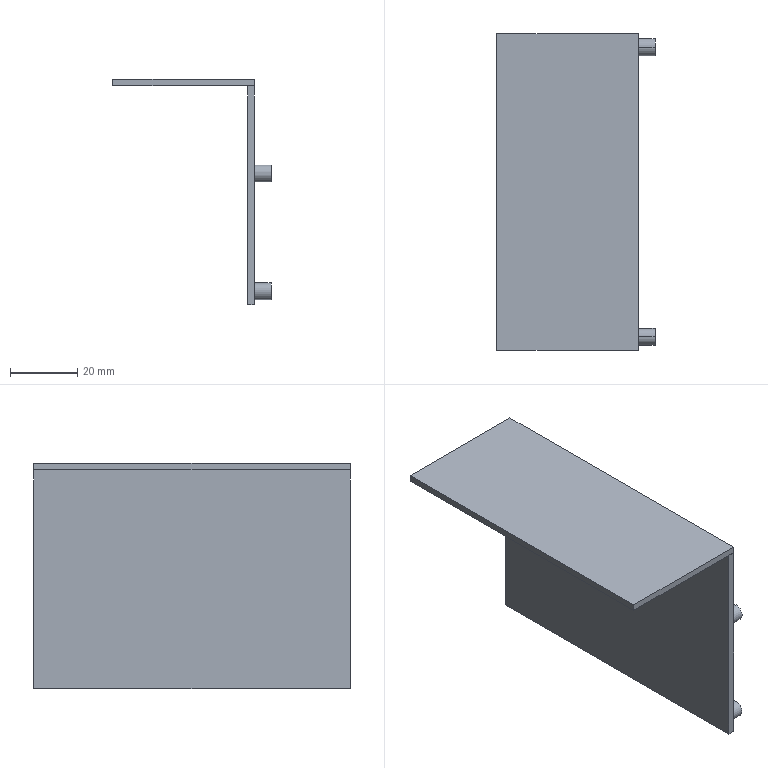Part | SolidWorks | features ICE 2, Cut 1, Extrusion 1, HoleWzd 1 | 6 solids | 48 faces | box 47 x 94 x 67 mm | volume 20411 mm3 | plane 24 | cylinder 24 | commonest cylinder face diameters 2.5 x16 5 x8
STEP:
#1=CARTESIAN_POINT('',(21.,-47.,0.));
#2=VERTEX_POINT('',#1);
#3=CARTESIAN_POINT('',(21.,47.,0.));
#4=VERTEX_POINT('',#3);
#5=CARTESIAN_POINT('',(21.,-47.,0.));
#6=DIRECTION('',(0.,1.,0.));
#7=VECTOR('',#6,1000.);
#8=LINE('',#5,#7);
#9=EDGE_CURVE('',#2,#4,#8,.T.);
#10=ORIENTED_EDGE('',*,*,#9,.T.);
#11=CARTESIAN_POINT('',(21.,47.,2.));
#12=VERTEX_POINT('',#11);
#13=CARTESIAN_POINT('',(21.,47.,2.));
#14=DIRECTION('',(0.,0.,-1.));
#15=VECTOR('',#14,1000.);
#16=LINE('',#13,#15);
#17=EDGE_CURVE('',#12,#4,#16,.T.);
#18=ORIENTED_EDGE('',*,*,#17,.F.);
#19=CARTESIAN_POINT('',(21.,-47.,2.));
#20=VERTEX_POINT('',#19);
#21=CARTESIAN_POINT('',(21.,-47.,2.));
#22=DIRECTION('',(0.,1.,0.));
#23=VECTOR('',#22,1000.);
#24=LINE('',#21,#23);
#25=EDGE_CURVE('',#20,#12,#24,.T.);
#26=ORIENTED_EDGE('',*,*,#25,.F.);
#27=CARTESIAN_POINT('',(21.,-47.,2.));
#28=DIRECTION('',(0.,0.,-1.));
#29=VECTOR('',#28,1000.);
#30=LINE('',#27,#29);
#31=EDGE_CURVE('',#20,#2,#30,.T.);
#32=ORIENTED_EDGE('',*,*,#31,.T.);
#33=EDGE_LOOP('',(#10,#18,#26,#32));
#34=FACE_OUTER_BOUND('',#33,.T.);
#35=CARTESIAN_POINT('',(21.,-47.,2.));
#36=DIRECTION('',(-1.,0.,0.));
#37=DIRECTION('',(0.,0.,1.));
#38=AXIS2_PLACEMENT_3D('',#35,#36,#37);
#39=PLANE('',#38);
#40=ADVANCED_FACE('',(#34),#39,.F.);
#41=CARTESIAN_POINT('',(-21.,47.,0.));
#42=VERTEX_POINT('',#41);
#43=CARTESIAN_POINT('',(-21.,47.,0.));
#44=DIRECTION('',(-1.,0.,0.));
#45=VECTOR('',#44,1000.);
#46=LINE('',#43,#45);
#47=EDGE_CURVE('',#4,#42,#46,.T.);
#48=ORIENTED_EDGE('',*,*,#47,.T.);
#49=CARTESIAN_POINT('',(-21.,47.,2.));
#50=VERTEX_POINT('',#49);
#51=CARTESIAN_POINT('',(-21.,47.,2.));
#52=DIRECTION('',(0.,0.,-1.));
#53=VECTOR('',#52,1000.);
#54=LINE('',#51,#53);
#55=EDGE_CURVE('',#50,#42,#54,.T.);
#56=ORIENTED_EDGE('',*,*,#55,.F.);
#57=CARTESIAN_POINT('',(-21.,47.,2.));
#58=DIRECTION('',(-1.,0.,0.));
#59=VECTOR('',#58,1000.);
#60=LINE('',#57,#59);
#61=EDGE_CURVE('',#12,#50,#60,.T.);
#62=ORIENTED_EDGE('',*,*,#61,.F.);
#63=ORIENTED_EDGE('',*,*,#17,.T.);
#64=EDGE_LOOP('',(#48,#56,#62,#63));
#65=FACE_OUTER_BOUND('',#64,.T.);
#66=CARTESIAN_POINT('',(-21.,47.,2.));
#67=DIRECTION('',(0.,-1.,0.));
#68=DIRECTION('',(0.,0.,-1.));
#69=AXIS2_PLACEMENT_3D('',#66,#67,#68);
#70=PLANE('',#69);
#71=ADVANCED_FACE('',(#65),#70,.F.);
#72=CARTESIAN_POINT('',(-21.,-47.,0.));
#73=VERTEX_POINT('',#72);
#74=CARTESIAN_POINT('',(-21.,-47.,0.));
#75=DIRECTION('',(0.,-1.,0.));
#76=VECTOR('',#75,1000.);
#77=LINE('',#74,#76);
#78=EDGE_CURVE('',#42,#73,#77,.T.);
#79=ORIENTED_EDGE('',*,*,#78,.T.);
#80=CARTESIAN_POINT('',(-21.,-47.,2.));
#81=VERTEX_POINT('',#80);
#82=CARTESIAN_POINT('',(-21.,-47.,2.));
#83=DIRECTION('',(0.,0.,-1.));
#84=VECTOR('',#83,1000.);
#85=LINE('',#82,#84);
#86=EDGE_CURVE('',#81,#73,#85,.T.);
#87=ORIENTED_EDGE('',*,*,#86,.F.);
#88=CARTESIAN_POINT('',(-21.,-47.,2.));
#89=DIRECTION('',(0.,-1.,0.));
#90=VECTOR('',#89,1000.);
#91=LINE('',#88,#90);
#92=EDGE_CURVE('',#50,#81,#91,.T.);
#93=ORIENTED_EDGE('',*,*,#92,.F.);
#94=ORIENTED_EDGE('',*,*,#55,.T.);
#95=EDGE_LOOP('',(#79,#87,#93,#94));
#96=FACE_OUTER_BOUND('',#95,.T.);
#97=CARTESIAN_POINT('',(-21.,-47.,2.));
#98=DIRECTION('',(1.,0.,0.));
#99=DIRECTION('',(0.,0.,-1.));
#100=AXIS2_PLACEMENT_3D('',#97,#98,#99);
#101=PLANE('',#100);
#102=ADVANCED_FACE('',(#96),#101,.F.);
#103=CARTESIAN_POINT('',(-21.,-47.,0.));
#104=DIRECTION('',(1.,0.,0.));
#105=VECTOR('',#104,1000.);
#106=LINE('',#103,#105);
#107=EDGE_CURVE('',#73,#2,#106,.T.);
#108=ORIENTED_EDGE('',*,*,#107,.T.);
#109=ORIENTED_EDGE('',*,*,#31,.F.);
#110=CARTESIAN_POINT('',(-21.,-47.,2.));
#111=DIRECTION('',(1.,0.,0.));
#112=VECTOR('',#111,1000.);
#113=LINE('',#110,#112);
#114=EDGE_CURVE('',#81,#20,#113,.T.);
#115=ORIENTED_EDGE('',*,*,#114,.F.);
#116=ORIENTED_EDGE('',*,*,#86,.T.);
#117=EDGE_LOOP('',(#108,#109,#115,#116));
#118=FACE_OUTER_BOUND('',#117,.T.);
#119=CARTESIAN_POINT('',(-21.,-47.,2.));
#120=DIRECTION('',(0.,1.,0.));
#121=DIRECTION('',(0.,0.,1.));
#122=AXIS2_PLACEMENT_3D('',#119,#120,#121);
#123=PLANE('',#122);
#124=ADVANCED_FACE('',(#118),#123,.F.);
#125=ORIENTED_EDGE('',*,*,#25,.T.);
#126=ORIENTED_EDGE('',*,*,#61,.T.);
#127=ORIENTED_EDGE('',*,*,#92,.T.);
#128=ORIENTED_EDGE('',*,*,#114,.T.);
#129=EDGE_LOOP('',(#125,#126,#127,#128));
#130=FACE_OUTER_BOUND('',#129,.T.);
#131=CARTESIAN_POINT('',(0.,0.,2.));
#132=DIRECTION('',(0.,0.,-1.));
#133=DIRECTION('',(-1.,0.,0.));
#134=AXIS2_PLACEMENT_3D('',#131,#132,#133);
#135=PLANE('',#134);
#136=ADVANCED_FACE('',(#130),#135,.F.);
#137=ORIENTED_EDGE('',*,*,#9,.F.);
#138=ORIENTED_EDGE('',*,*,#107,.F.);
#139=ORIENTED_EDGE('',*,*,#78,.F.);
#140=ORIENTED_EDGE('',*,*,#47,.F.);
#141=EDGE_LOOP('',(#137,#138,#139,#140));
#142=FACE_OUTER_BOUND('',#141,.T.);
#143=CARTESIAN_POINT('',(0.,0.,0.));
#144=DIRECTION('',(0.,0.,-1.));
#145=DIRECTION('',(-1.,0.,0.));
#146=AXIS2_PLACEMENT_3D('',#143,#144,#145);
#147=PLANE('',#146);
#148=ADVANCED_FACE('',(#142),#147,.T.);
#149=CLOSED_SHELL('',(#40,#71,#102,#124,#136,#148));
#150=MANIFOLD_SOLID_BREP('',#149);
#151=CARTESIAN_POINT('',(20.999,43.,-24.75));
#152=VERTEX_POINT('',#151);
#153=CARTESIAN_POINT('',(20.999,43.,-27.25));
#154=VERTEX_POINT('',#153);
#155=CARTESIAN_POINT('',(20.999,43.,-26.));
#156=DIRECTION('',(1.,0.,0.));
#157=DIRECTION('',(0.,0.,-1.));
#158=AXIS2_PLACEMENT_3D('',#155,#156,#157);
#159=CIRCLE('',#158,1.25);
#160=EDGE_CURVE('',#152,#154,#159,.T.);
#161=ORIENTED_EDGE('',*,*,#160,.F.);
#162=CARTESIAN_POINT('',(21.,43.,-24.75));
#163=VERTEX_POINT('',#162);
#164=CARTESIAN_POINT('',(26.,43.,-24.75));
#165=DIRECTION('',(1.,0.,0.));
#166=VECTOR('',#165,1000.);
#167=LINE('',#164,#166);
#168=EDGE_CURVE('',#152,#163,#167,.T.);
#169=ORIENTED_EDGE('',*,*,#168,.T.);
#170=CARTESIAN_POINT('',(21.,43.,-27.25));
#171=VERTEX_POINT('',#170);
#172=CARTESIAN_POINT('',(21.,43.,-26.));
#173=DIRECTION('',(-1.,0.,0.));
#174=DIRECTION('',(0.,0.,1.));
#175=AXIS2_PLACEMENT_3D('',#172,#173,#174);
#176=CIRCLE('',#175,1.25);
#177=EDGE_CURVE('',#171,#163,#176,.T.);
#178=ORIENTED_EDGE('',*,*,#177,.F.);
#179=CARTESIAN_POINT('',(26.,43.,-27.25));
#180=DIRECTION('',(1.,0.,0.));
#181=VECTOR('',#180,1000.);
#182=LINE('',#179,#181);
#183=EDGE_CURVE('',#154,#171,#182,.T.);
#184=ORIENTED_EDGE('',*,*,#183,.F.);
#185=EDGE_LOOP('',(#161,#169,#178,#184));
#186=FACE_OUTER_BOUND('',#185,.T.);
#187=CARTESIAN_POINT('',(26.,43.,-26.));
#188=DIRECTION('',(1.,0.,0.));
#189=DIRECTION('',(0.,0.,-1.));
#190=AXIS2_PLACEMENT_3D('',#187,#188,#189);
#191=CYLINDRICAL_SURFACE('',#190,1.25);
#192=ADVANCED_FACE('',(#186),#191,.F.);
#193=CARTESIAN_POINT('',(20.999,43.,-59.75));
#194=VERTEX_POINT('',#193);
#195=CARTESIAN_POINT('',(20.999,43.,-62.25));
#196=VERTEX_POINT('',#195);
#197=CARTESIAN_POINT('',(20.999,43.,-61.));
#198=DIRECTION('',(1.,0.,0.));
#199=DIRECTION('',(0.,0.,-1.));
#200=AXIS2_PLACEMENT_3D('',#197,#198,#199);
#201=CIRCLE('',#200,1.25);
#202=EDGE_CURVE('',#194,#196,#201,.T.);
#203=ORIENTED_EDGE('',*,*,#202,.F.);
#204=CARTESIAN_POINT('',(21.,43.,-59.75));
#205=VERTEX_POINT('',#204);
#206=CARTESIAN_POINT('',(26.,43.,-59.75));
#207=DIRECTION('',(1.,0.,0.));
#208=VECTOR('',#207,1000.);
#209=LINE('',#206,#208);
#210=EDGE_CURVE('',#194,#205,#209,.T.);
#211=ORIENTED_EDGE('',*,*,#210,.T.);
#212=CARTESIAN_POINT('',(21.,43.,-62.25));
#213=VERTEX_POINT('',#212);
#214=CARTESIAN_POINT('',(21.,43.,-61.));
#215=DIRECTION('',(-1.,0.,0.));
#216=DIRECTION('',(0.,0.,1.));
#217=AXIS2_PLACEMENT_3D('',#214,#215,#216);
#218=CIRCLE('',#217,1.25);
#219=EDGE_CURVE('',#213,#205,#218,.T.);
#220=ORIENTED_EDGE('',*,*,#219,.F.);
#221=CARTESIAN_POINT('',(26.,43.,-62.25));
#222=DIRECTION('',(1.,0.,0.));
#223=VECTOR('',#222,1000.);
#224=LINE('',#221,#223);
#225=EDGE_CURVE('',#196,#213,#224,.T.);
#226=ORIENTED_EDGE('',*,*,#225,.F.);
#227=EDGE_LOOP('',(#203,#211,#220,#226));
#228=FACE_OUTER_BOUND('',#227,.T.);
#229=CARTESIAN_POINT('',(26.,43.,-61.));
#230=DIRECTION('',(1.,0.,0.));
#231=DIRECTION('',(0.,0.,-1.));
#232=AXIS2_PLACEMENT_3D('',#229,#230,#231);
#233=CYLINDRICAL_SURFACE('',#232,1.25);
#234=ADVANCED_FACE('',(#228),#233,.F.);
#235=CARTESIAN_POINT('',(20.999,-43.,-24.75));
#236=VERTEX_POINT('',#235);
#237=CARTESIAN_POINT('',(20.999,-43.,-27.25));
#238=VERTEX_POINT('',#237);
#239=CARTESIAN_POINT('',(20.999,-43.,-26.));
#240=DIRECTION('',(1.,0.,0.));
#241=DIRECTION('',(0.,0.,-1.));
#242=AXIS2_PLACEMENT_3D('',#239,#240,#241);
#243=CIRCLE('',#242,1.25);
#244=EDGE_CURVE('',#236,#238,#243,.T.);
#245=ORIENTED_EDGE('',*,*,#244,.F.);
#246=CARTESIAN_POINT('',(21.,-43.,-24.75));
#247=VERTEX_POINT('',#246);
#248=CARTESIAN_POINT('',(26.,-43.,-24.75));
#249=DIRECTION('',(1.,0.,0.));
#250=VECTOR('',#249,1000.);
#251=LINE('',#248,#250);
#252=EDGE_CURVE('',#236,#247,#251,.T.);
#253=ORIENTED_EDGE('',*,*,#252,.T.);
#254=CARTESIAN_POINT('',(21.,-43.,-27.25));
#255=VERTEX_POINT('',#254);
#256=CARTESIAN_POINT('',(21.,-43.,-26.));
#257=DIRECTION('',(-1.,0.,0.));
#258=DIRECTION('',(0.,0.,1.));
#259=AXIS2_PLACEMENT_3D('',#256,#257,#258);
#260=CIRCLE('',#259,1.25);
#261=EDGE_CURVE('',#255,#247,#260,.T.);
#262=ORIENTED_EDGE('',*,*,#261,.F.);
#263=CARTESIAN_POINT('',(26.,-43.,-27.25));
#264=DIRECTION('',(1.,0.,0.));
#265=VECTOR('',#264,1000.);
#266=LINE('',#263,#265);
#267=EDGE_CURVE('',#238,#255,#266,.T.);
#268=ORIENTED_EDGE('',*,*,#267,.F.);
#269=EDGE_LOOP('',(#245,#253,#262,#268));
#270=FACE_OUTER_BOUND('',#269,.T.);
#271=CARTESIAN_POINT('',(26.,-43.,-26.));
#272=DIRECTION('',(1.,0.,0.));
#273=DIRECTION('',(0.,0.,-1.));
#274=AXIS2_PLACEMENT_3D('',#271,#272,#273);
#275=CYLINDRICAL_SURFACE('',#274,1.25);
#276=ADVANCED_FACE('',(#270),#275,.F.);
#277=CARTESIAN_POINT('',(20.999,-43.,-59.75));
#278=VERTEX_POINT('',#277);
#279=CARTESIAN_POINT('',(20.999,-43.,-62.25));
#280=VERTEX_POINT('',#279);
#281=CARTESIAN_POINT('',(20.999,-43.,-61.));
#282=DIRECTION('',(1.,0.,0.));
#283=DIRECTION('',(0.,0.,-1.));
#284=AXIS2_PLACEMENT_3D('',#281,#282,#283);
#285=CIRCLE('',#284,1.25);
#286=EDGE_CURVE('',#278,#280,#285,.T.);
#287=ORIENTED_EDGE('',*,*,#286,.F.);
#288=CARTESIAN_POINT('',(21.,-43.,-59.75));
#289=VERTEX_POINT('',#288);
#290=CARTESIAN_POINT('',(26.,-43.,-59.75));
#291=DIRECTION('',(1.,0.,0.));
#292=VECTOR('',#291,1000.);
#293=LINE('',#290,#292);
#294=EDGE_CURVE('',#278,#289,#293,.T.);
#295=ORIENTED_EDGE('',*,*,#294,.T.);
#296=CARTESIAN_POINT('',(21.,-43.,-62.25));
#297=VERTEX_POINT('',#296);
#298=CARTESIAN_POINT('',(21.,-43.,-61.));
#299=DIRECTION('',(-1.,0.,0.));
#300=DIRECTION('',(0.,0.,1.));
#301=AXIS2_PLACEMENT_3D('',#298,#299,#300);
#302=CIRCLE('',#301,1.25);
#303=EDGE_CURVE('',#297,#289,#302,.T.);
#304=ORIENTED_EDGE('',*,*,#303,.F.);
#305=CARTESIAN_POINT('',(26.,-43.,-62.25));
#306=DIRECTION('',(1.,0.,0.));
#307=VECTOR('',#306,1000.);
#308=LINE('',#305,#307);
#309=EDGE_CURVE('',#280,#297,#308,.T.);
#310=ORIENTED_EDGE('',*,*,#309,.F.);
#311=EDGE_LOOP('',(#287,#295,#304,#310));
#312=FACE_OUTER_BOUND('',#311,.T.);
#313=CARTESIAN_POINT('',(26.,-43.,-61.));
#314=DIRECTION('',(1.,0.,0.));
#315=DIRECTION('',(0.,0.,-1.));
#316=AXIS2_PLACEMENT_3D('',#313,#314,#315);
#317=CYLINDRICAL_SURFACE('',#316,1.25);
#318=ADVANCED_FACE('',(#312),#317,.F.);
#319=ORIENTED_EDGE('',*,*,#177,.T.);
#320=CARTESIAN_POINT('',(21.,43.,-26.));
#321=DIRECTION('',(-1.,0.,0.));
#322=DIRECTION('',(0.,0.,1.));
#323=AXIS2_PLACEMENT_3D('',#320,#321,#322);
#324=CIRCLE('',#323,1.25);
#325=EDGE_CURVE('',#163,#171,#324,.T.);
#326=ORIENTED_EDGE('',*,*,#325,.T.);
#327=EDGE_LOOP('',(#319,#326));
#328=FACE_BOUND('',#327,.T.);
#329=ORIENTED_EDGE('',*,*,#219,.T.);
#330=CARTESIAN_POINT('',(21.,43.,-61.));
#331=DIRECTION('',(-1.,0.,0.));
#332=DIRECTION('',(0.,0.,1.));
#333=AXIS2_PLACEMENT_3D('',#330,#331,#332);
#334=CIRCLE('',#333,1.25);
#335=EDGE_CURVE('',#205,#213,#334,.T.);
#336=ORIENTED_EDGE('',*,*,#335,.T.);
#337=EDGE_LOOP('',(#329,#336));
#338=FACE_BOUND('',#337,.T.);
#339=ORIENTED_EDGE('',*,*,#261,.T.);
#340=CARTESIAN_POINT('',(21.,-43.,-26.));
#341=DIRECTION('',(-1.,0.,0.));
#342=DIRECTION('',(0.,0.,1.));
#343=AXIS2_PLACEMENT_3D('',#340,#341,#342);
#344=CIRCLE('',#343,1.25);
#345=EDGE_CURVE('',#247,#255,#344,.T.);
#346=ORIENTED_EDGE('',*,*,#345,.T.);
#347=EDGE_LOOP('',(#339,#346));
#348=FACE_BOUND('',#347,.T.);
#349=ORIENTED_EDGE('',*,*,#303,.T.);
#350=CARTESIAN_POINT('',(21.,-43.,-61.));
#351=DIRECTION('',(-1.,0.,0.));
#352=DIRECTION('',(0.,0.,1.));
#353=AXIS2_PLACEMENT_3D('',#350,#351,#352);
#354=CIRCLE('',#353,1.25);
#355=EDGE_CURVE('',#289,#297,#354,.T.);
#356=ORIENTED_EDGE('',*,*,#355,.T.);
#357=EDGE_LOOP('',(#349,#356));
#358=FACE_BOUND('',#357,.T.);
#359=CARTESIAN_POINT('',(21.,47.,0.));
#360=VERTEX_POINT('',#359);
#361=CARTESIAN_POINT('',(21.,-47.,0.));
#362=VERTEX_POINT('',#361);
#363=CARTESIAN_POINT('',(21.,47.,0.));
#364=DIRECTION('',(0.,-1.,0.));
#365=VECTOR('',#364,1000.);
#366=LINE('',#363,#365);
#367=EDGE_CURVE('',#360,#362,#366,.T.);
#368=ORIENTED_EDGE('',*,*,#367,.T.);
#369=CARTESIAN_POINT('',(21.,-47.,-65.));
#370=VERTEX_POINT('',#369);
#371=CARTESIAN_POINT('',(21.,-47.,-65.));
#372=DIRECTION('',(0.,0.,1.));
#373=VECTOR('',#372,1000.);
#374=LINE('',#371,#373);
#375=EDGE_CURVE('',#370,#362,#374,.T.);
#376=ORIENTED_EDGE('',*,*,#375,.F.);
#377=CARTESIAN_POINT('',(21.,47.,-65.));
#378=VERTEX_POINT('',#377);
#379=CARTESIAN_POINT('',(21.,47.,-65.));
#380=DIRECTION('',(0.,-1.,0.));
#381=VECTOR('',#380,1000.);
#382=LINE('',#379,#381);
#383=EDGE_CURVE('',#378,#370,#382,.T.);
#384=ORIENTED_EDGE('',*,*,#383,.F.);
#385=CARTESIAN_POINT('',(21.,47.,-65.));
#386=DIRECTION('',(0.,0.,1.));
#387=VECTOR('',#386,1000.);
#388=LINE('',#385,#387);
#389=EDGE_CURVE('',#378,#360,#388,.T.);
#390=ORIENTED_EDGE('',*,*,#389,.T.);
#391=EDGE_LOOP('',(#368,#376,#384,#390));
#392=FACE_OUTER_BOUND('',#391,.T.);
#393=CARTESIAN_POINT('',(21.,47.,-65.));
#394=DIRECTION('',(-1.,0.,0.));
#395=DIRECTION('',(0.,0.,1.));
#396=AXIS2_PLACEMENT_3D('',#393,#394,#395);
#397=PLANE('',#396);
#398=ADVANCED_FACE('',(#328,#338,#348,#358,#392),#397,.F.);
#399=CARTESIAN_POINT('',(19.,-47.,0.));
#400=VERTEX_POINT('',#399);
#401=CARTESIAN_POINT('',(21.,-47.,0.));
#402=DIRECTION('',(-1.,0.,0.));
#403=VECTOR('',#402,1000.);
#404=LINE('',#401,#403);
#405=EDGE_CURVE('',#362,#400,#404,.T.);
#406=ORIENTED_EDGE('',*,*,#405,.T.);
#407=CARTESIAN_POINT('',(19.,-47.,-65.));
#408=VERTEX_POINT('',#407);
#409=CARTESIAN_POINT('',(19.,-47.,-65.));
#410=DIRECTION('',(0.,0.,1.));
#411=VECTOR('',#410,1000.);
#412=LINE('',#409,#411);
#413=EDGE_CURVE('',#408,#400,#412,.T.);
#414=ORIENTED_EDGE('',*,*,#413,.F.);
#415=CARTESIAN_POINT('',(21.,-47.,-65.));
#416=DIRECTION('',(-1.,0.,0.));
#417=VECTOR('',#416,1000.);
#418=LINE('',#415,#417);
#419=EDGE_CURVE('',#370,#408,#418,.T.);
#420=ORIENTED_EDGE('',*,*,#419,.F.);
#421=ORIENTED_EDGE('',*,*,#375,.T.);
#422=EDGE_LOOP('',(#406,#414,#420,#421));
#423=FACE_OUTER_BOUND('',#422,.T.);
#424=CARTESIAN_POINT('',(21.,-47.,-65.));
#425=DIRECTION('',(0.,1.,0.));
#426=DIRECTION('',(0.,0.,1.));
#427=AXIS2_PLACEMENT_3D('',#424,#425,#426);
#428=PLANE('',#427);
#429=ADVANCED_FACE('',(#423),#428,.F.);
#430=CARTESIAN_POINT('',(19.,47.,0.));
#431=VERTEX_POINT('',#430);
#432=CARTESIAN_POINT('',(19.,47.,0.));
#433=DIRECTION('',(0.,1.,0.));
#434=VECTOR('',#433,1000.);
#435=LINE('',#432,#434);
#436=EDGE_CURVE('',#400,#431,#435,.T.);
#437=ORIENTED_EDGE('',*,*,#436,.T.);
#438=CARTESIAN_POINT('',(19.,47.,-65.));
#439=VERTEX_POINT('',#438);
#440=CARTESIAN_POINT('',(19.,47.,-65.));
#441=DIRECTION('',(0.,0.,1.));
#442=VECTOR('',#441,1000.);
#443=LINE('',#440,#442);
#444=EDGE_CURVE('',#439,#431,#443,.T.);
#445=ORIENTED_EDGE('',*,*,#444,.F.);
#446=CARTESIAN_POINT('',(19.,47.,-65.));
#447=DIRECTION('',(0.,1.,0.));
#448=VECTOR('',#447,1000.);
#449=LINE('',#446,#448);
#450=EDGE_CURVE('',#408,#439,#449,.T.);
#451=ORIENTED_EDGE('',*,*,#450,.F.);
#452=ORIENTED_EDGE('',*,*,#413,.T.);
#453=EDGE_LOOP('',(#437,#445,#451,#452));
#454=FACE_OUTER_BOUND('',#453,.T.);
#455=CARTESIAN_POINT('',(19.,47.,-65.));
#456=DIRECTION('',(1.,0.,0.));
#457=DIRECTION('',(0.,1.,0.));
#458=AXIS2_PLACEMENT_3D('',#455,#456,#457);
#459=PLANE('',#458);
#460=ADVANCED_FACE('',(#454),#459,.F.);
#461=CARTESIAN_POINT('',(21.,47.,0.));
#462=DIRECTION('',(1.,0.,0.));
#463=VECTOR('',#462,1000.);
#464=LINE('',#461,#463);
#465=EDGE_CURVE('',#431,#360,#464,.T.);
#466=ORIENTED_EDGE('',*,*,#465,.T.);
#467=ORIENTED_EDGE('',*,*,#389,.F.);
#468=CARTESIAN_POINT('',(21.,47.,-65.));
#469=DIRECTION('',(1.,0.,0.));
#470=VECTOR('',#469,1000.);
#471=LINE('',#468,#470);
#472=EDGE_CURVE('',#439,#378,#471,.T.);
#473=ORIENTED_EDGE('',*,*,#472,.F.);
#474=ORIENTED_EDGE('',*,*,#444,.T.);
#475=EDGE_LOOP('',(#466,#467,#473,#474));
#476=FACE_OUTER_BOUND('',#475,.T.);
#477=CARTESIAN_POINT('',(21.,47.,-65.));
#478=DIRECTION('',(0.,-1.,0.));
#479=DIRECTION('',(0.,0.,-1.));
#480=AXIS2_PLACEMENT_3D('',#477,#478,#479);
#481=PLANE('',#480);
#482=ADVANCED_FACE('',(#476),#481,.F.);
#483=ORIENTED_EDGE('',*,*,#383,.T.);
#484=ORIENTED_EDGE('',*,*,#419,.T.);
#485=ORIENTED_EDGE('',*,*,#450,.T.);
#486=ORIENTED_EDGE('',*,*,#472,.T.);
#487=EDGE_LOOP('',(#483,#484,#485,#486));
#488=FACE_OUTER_BOUND('',#487,.T.);
#489=CARTESIAN_POINT('',(0.,0.,-65.));
#490=DIRECTION('',(0.,0.,-1.));
#491=DIRECTION('',(-1.,0.,0.));
#492=AXIS2_PLACEMENT_3D('',#489,#490,#491);
#493=PLANE('',#492);
#494=ADVANCED_FACE('',(#488),#493,.T.);
#495=ORIENTED_EDGE('',*,*,#367,.F.);
#496=ORIENTED_EDGE('',*,*,#465,.F.);
#497=ORIENTED_EDGE('',*,*,#436,.F.);
#498=ORIENTED_EDGE('',*,*,#405,.F.);
#499=EDGE_LOOP('',(#495,#496,#497,#498));
#500=FACE_OUTER_BOUND('',#499,.T.);
#501=CARTESIAN_POINT('',(0.,0.,0.));
#502=DIRECTION('',(0.,0.,-1.));
#503=DIRECTION('',(-1.,0.,0.));
#504=AXIS2_PLACEMENT_3D('',#501,#502,#503);
#505=PLANE('',#504);
#506=ADVANCED_FACE('',(#500),#505,.F.);
#507=ORIENTED_EDGE('',*,*,#294,.F.);
#508=CARTESIAN_POINT('',(20.999,-43.,-61.));
#509=DIRECTION('',(1.,0.,0.));
#510=DIRECTION('',(0.,0.,-1.));
#511=AXIS2_PLACEMENT_3D('',#508,#509,#510);
#512=CIRCLE('',#511,1.25);
#513=EDGE_CURVE('',#280,#278,#512,.T.);
#514=ORIENTED_EDGE('',*,*,#513,.F.);
#515=ORIENTED_EDGE('',*,*,#309,.T.);
#516=ORIENTED_EDGE('',*,*,#355,.F.);
#517=EDGE_LOOP('',(#507,#514,#515,#516));
#518=FACE_OUTER_BOUND('',#517,.T.);
#519=CARTESIAN_POINT('',(26.,-43.,-61.));
#520=DIRECTION('',(1.,0.,0.));
#521=DIRECTION('',(0.,0.,-1.));
#522=AXIS2_PLACEMENT_3D('',#519,#520,#521);
#523=CYLINDRICAL_SURFACE('',#522,1.25);
#524=ADVANCED_FACE('',(#518),#523,.F.);
#525=ORIENTED_EDGE('',*,*,#513,.T.);
#526=ORIENTED_EDGE('',*,*,#286,.T.);
#527=EDGE_LOOP('',(#525,#526));
#528=FACE_OUTER_BOUND('',#527,.T.);
#529=CARTESIAN_POINT('',(20.999,-43.,-61.));
#530=DIRECTION('',(-1.,0.,0.));
#531=DIRECTION('',(0.,0.,1.));
#532=AXIS2_PLACEMENT_3D('',#529,#530,#531);
#533=PLANE('',#532);
#534=ADVANCED_FACE('',(#528),#533,.F.);
#535=ORIENTED_EDGE('',*,*,#252,.F.);
#536=CARTESIAN_POINT('',(20.999,-43.,-26.));
#537=DIRECTION('',(1.,0.,0.));
#538=DIRECTION('',(0.,0.,-1.));
#539=AXIS2_PLACEMENT_3D('',#536,#537,#538);
#540=CIRCLE('',#539,1.25);
#541=EDGE_CURVE('',#238,#236,#540,.T.);
#542=ORIENTED_EDGE('',*,*,#541,.F.);
#543=ORIENTED_EDGE('',*,*,#267,.T.);
#544=ORIENTED_EDGE('',*,*,#345,.F.);
#545=EDGE_LOOP('',(#535,#542,#543,#544));
#546=FACE_OUTER_BOUND('',#545,.T.);
#547=CARTESIAN_POINT('',(26.,-43.,-26.));
#548=DIRECTION('',(1.,0.,0.));
#549=DIRECTION('',(0.,0.,-1.));
#550=AXIS2_PLACEMENT_3D('',#547,#548,#549);
#551=CYLINDRICAL_SURFACE('',#550,1.25);
#552=ADVANCED_FACE('',(#546),#551,.F.);
#553=ORIENTED_EDGE('',*,*,#541,.T.);
#554=ORIENTED_EDGE('',*,*,#244,.T.);
#555=EDGE_LOOP('',(#553,#554));
#556=FACE_OUTER_BOUND('',#555,.T.);
#557=CARTESIAN_POINT('',(20.999,-43.,-26.));
#558=DIRECTION('',(-1.,0.,0.));
#559=DIRECTION('',(0.,0.,1.));
#560=AXIS2_PLACEMENT_3D('',#557,#558,#559);
#561=PLANE('',#560);
#562=ADVANCED_FACE('',(#556),#561,.F.);
#563=ORIENTED_EDGE('',*,*,#210,.F.);
#564=CARTESIAN_POINT('',(20.999,43.,-61.));
#565=DIRECTION('',(1.,0.,0.));
#566=DIRECTION('',(0.,0.,-1.));
#567=AXIS2_PLACEMENT_3D('',#564,#565,#566);
#568=CIRCLE('',#567,1.25);
#569=EDGE_CURVE('',#196,#194,#568,.T.);
#570=ORIENTED_EDGE('',*,*,#569,.F.);
#571=ORIENTED_EDGE('',*,*,#225,.T.);
#572=ORIENTED_EDGE('',*,*,#335,.F.);
#573=EDGE_LOOP('',(#563,#570,#571,#572));
#574=FACE_OUTER_BOUND('',#573,.T.);
#575=CARTESIAN_POINT('',(26.,43.,-61.));
#576=DIRECTION('',(1.,0.,0.));
#577=DIRECTION('',(0.,0.,-1.));
#578=AXIS2_PLACEMENT_3D('',#575,#576,#577);
#579=CYLINDRICAL_SURFACE('',#578,1.25);
#580=ADVANCED_FACE('',(#574),#579,.F.);
#581=ORIENTED_EDGE('',*,*,#569,.T.);
#582=ORIENTED_EDGE('',*,*,#202,.T.);
#583=EDGE_LOOP('',(#581,#582));
#584=FACE_OUTER_BOUND('',#583,.T.);
#585=CARTESIAN_POINT('',(20.999,43.,-61.));
#586=DIRECTION('',(-1.,0.,0.));
#587=DIRECTION('',(0.,0.,1.));
#588=AXIS2_PLACEMENT_3D('',#585,#586,#587);
#589=PLANE('',#588);
#590=ADVANCED_FACE('',(#584),#589,.F.);
#591=ORIENTED_EDGE('',*,*,#168,.F.);
#592=CARTESIAN_POINT('',(20.999,43.,-26.));
#593=DIRECTION('',(1.,0.,0.));
#594=DIRECTION('',(0.,0.,-1.));
#595=AXIS2_PLACEMENT_3D('',#592,#593,#594);
#596=CIRCLE('',#595,1.25);
#597=EDGE_CURVE('',#154,#152,#596,.T.);
#598=ORIENTED_EDGE('',*,*,#597,.F.);
#599=ORIENTED_EDGE('',*,*,#183,.T.);
#600=ORIENTED_EDGE('',*,*,#325,.F.);
#601=EDGE_LOOP('',(#591,#598,#599,#600));
#602=FACE_OUTER_BOUND('',#601,.T.);
#603=CARTESIAN_POINT('',(26.,43.,-26.));
#604=DIRECTION('',(1.,0.,0.));
#605=DIRECTION('',(0.,0.,-1.));
#606=AXIS2_PLACEMENT_3D('',#603,#604,#605);
#607=CYLINDRICAL_SURFACE('',#606,1.25);
#608=ADVANCED_FACE('',(#602),#607,.F.);
#609=ORIENTED_EDGE('',*,*,#597,.T.);
#610=ORIENTED_EDGE('',*,*,#160,.T.);
#611=EDGE_LOOP('',(#609,#610));
#612=FACE_OUTER_BOUND('',#611,.T.);
#613=CARTESIAN_POINT('',(20.999,43.,-26.));
#614=DIRECTION('',(-1.,0.,0.));
#615=DIRECTION('',(0.,0.,1.));
#616=AXIS2_PLACEMENT_3D('',#613,#614,#615);
#617=PLANE('',#616);
#618=ADVANCED_FACE('',(#612),#617,.F.);
#619=CLOSED_SHELL('',(#192,#234,#276,#318,#398,#429,#460,#482,#494,#506,#524,#534,#552,#562,#580,#590,#608,#618));
#620=MANIFOLD_SOLID_BREP('',#619);
#621=CARTESIAN_POINT('',(21.,43.,-24.75));
#622=VERTEX_POINT('',#621);
#623=CARTESIAN_POINT('',(21.,43.,-27.25));
#624=VERTEX_POINT('',#623);
#625=CARTESIAN_POINT('',(21.,43.,-26.));
#626=DIRECTION('',(1.,0.,0.));
#627=DIRECTION('',(0.,0.,-1.));
#628=AXIS2_PLACEMENT_3D('',#625,#626,#627);
#629=CIRCLE('',#628,1.25);
#630=EDGE_CURVE('',#622,#624,#629,.T.);
#631=ORIENTED_EDGE('',*,*,#630,.F.);
#632=CARTESIAN_POINT('',(26.,43.,-24.75));
#633=VERTEX_POINT('',#632);
#634=CARTESIAN_POINT('',(26.,43.,-24.75));
#635=DIRECTION('',(1.,0.,0.));
#636=VECTOR('',#635,1000.);
#637=LINE('',#634,#636);
#638=EDGE_CURVE('',#622,#633,#637,.T.);
#639=ORIENTED_EDGE('',*,*,#638,.T.);
#640=CARTESIAN_POINT('',(26.,43.,-27.25));
#641=VERTEX_POINT('',#640);
#642=CARTESIAN_POINT('',(26.,43.,-26.));
#643=DIRECTION('',(1.,0.,0.));
#644=DIRECTION('',(0.,0.,-1.));
#645=AXIS2_PLACEMENT_3D('',#642,#643,#644);
#646=CIRCLE('',#645,1.25);
#647=EDGE_CURVE('',#633,#641,#646,.T.);
#648=ORIENTED_EDGE('',*,*,#647,.T.);
#649=CARTESIAN_POINT('',(26.,43.,-27.25));
#650=DIRECTION('',(1.,0.,0.));
#651=VECTOR('',#650,1000.);
#652=LINE('',#649,#651);
#653=EDGE_CURVE('',#624,#641,#652,.T.);
#654=ORIENTED_EDGE('',*,*,#653,.F.);
#655=EDGE_LOOP('',(#631,#639,#648,#654));
#656=FACE_OUTER_BOUND('',#655,.T.);
#657=CARTESIAN_POINT('',(26.,43.,-26.));
#658=DIRECTION('',(1.,0.,0.));
#659=DIRECTION('',(0.,0.,-1.));
#660=AXIS2_PLACEMENT_3D('',#657,#658,#659);
#661=CYLINDRICAL_SURFACE('',#660,1.25);
#662=ADVANCED_FACE('',(#656),#661,.F.);
#663=CARTESIAN_POINT('',(26.,43.,-28.5));
#664=VERTEX_POINT('',#663);
#665=CARTESIAN_POINT('',(26.,43.,-23.5));
#666=VERTEX_POINT('',#665);
#667=CARTESIAN_POINT('',(26.,43.,-26.));
#668=DIRECTION('',(1.,0.,0.));
#669=DIRECTION('',(0.,0.,-1.));
#670=AXIS2_PLACEMENT_3D('',#667,#668,#669);
#671=CIRCLE('',#670,2.5);
#672=EDGE_CURVE('',#664,#666,#671,.T.);
#673=ORIENTED_EDGE('',*,*,#672,.F.);
#674=CARTESIAN_POINT('',(21.,43.,-28.5));
#675=VERTEX_POINT('',#674);
#676=CARTESIAN_POINT('',(26.,43.,-28.5));
#677=DIRECTION('',(-1.,0.,0.));
#678=VECTOR('',#677,1000.);
#679=LINE('',#676,#678);
#680=EDGE_CURVE('',#664,#675,#679,.T.);
#681=ORIENTED_EDGE('',*,*,#680,.T.);
#682=CARTESIAN_POINT('',(21.,43.,-23.5));
#683=VERTEX_POINT('',#682);
#684=CARTESIAN_POINT('',(21.,43.,-26.));
#685=DIRECTION('',(1.,0.,0.));
#686=DIRECTION('',(0.,0.,-1.));
#687=AXIS2_PLACEMENT_3D('',#684,#685,#686);
#688=CIRCLE('',#687,2.5);
#689=EDGE_CURVE('',#675,#683,#688,.T.);
#690=ORIENTED_EDGE('',*,*,#689,.T.);
#691=CARTESIAN_POINT('',(26.,43.,-23.5));
#692=DIRECTION('',(-1.,0.,0.));
#693=VECTOR('',#692,1000.);
#694=LINE('',#691,#693);
#695=EDGE_CURVE('',#666,#683,#694,.T.);
#696=ORIENTED_EDGE('',*,*,#695,.F.);
#697=EDGE_LOOP('',(#673,#681,#690,#696));
#698=FACE_OUTER_BOUND('',#697,.T.);
#699=CARTESIAN_POINT('',(26.,43.,-26.));
#700=DIRECTION('',(-1.,0.,0.));
#701=DIRECTION('',(0.,0.,1.));
#702=AXIS2_PLACEMENT_3D('',#699,#700,#701);
#703=CYLINDRICAL_SURFACE('',#702,2.5);
#704=ADVANCED_FACE('',(#698),#703,.T.);
#705=ORIENTED_EDGE('',*,*,#680,.F.);
#706=CARTESIAN_POINT('',(26.,43.,-26.));
#707=DIRECTION('',(1.,0.,0.));
#708=DIRECTION('',(0.,0.,-1.));
#709=AXIS2_PLACEMENT_3D('',#706,#707,#708);
#710=CIRCLE('',#709,2.5);
#711=EDGE_CURVE('',#666,#664,#710,.T.);
#712=ORIENTED_EDGE('',*,*,#711,.F.);
#713=ORIENTED_EDGE('',*,*,#695,.T.);
#714=CARTESIAN_POINT('',(21.,43.,-26.));
#715=DIRECTION('',(1.,0.,0.));
#716=DIRECTION('',(0.,0.,-1.));
#717=AXIS2_PLACEMENT_3D('',#714,#715,#716);
#718=CIRCLE('',#717,2.5);
#719=EDGE_CURVE('',#683,#675,#718,.T.);
#720=ORIENTED_EDGE('',*,*,#719,.T.);
#721=EDGE_LOOP('',(#705,#712,#713,#720));
#722=FACE_OUTER_BOUND('',#721,.T.);
#723=CARTESIAN_POINT('',(26.,43.,-26.));
#724=DIRECTION('',(-1.,0.,0.));
#725=DIRECTION('',(0.,0.,1.));
#726=AXIS2_PLACEMENT_3D('',#723,#724,#725);
#727=CYLINDRICAL_SURFACE('',#726,2.5);
#728=ADVANCED_FACE('',(#722),#727,.T.);
#729=CARTESIAN_POINT('',(26.,43.,-26.));
#730=DIRECTION('',(1.,0.,0.));
#731=DIRECTION('',(0.,0.,-1.));
#732=AXIS2_PLACEMENT_3D('',#729,#730,#731);
#733=CIRCLE('',#732,1.25);
#734=EDGE_CURVE('',#641,#633,#733,.T.);
#735=ORIENTED_EDGE('',*,*,#734,.F.);
#736=ORIENTED_EDGE('',*,*,#647,.F.);
#737=EDGE_LOOP('',(#735,#736));
#738=FACE_BOUND('',#737,.T.);
#739=ORIENTED_EDGE('',*,*,#711,.T.);
#740=ORIENTED_EDGE('',*,*,#672,.T.);
#741=EDGE_LOOP('',(#739,#740));
#742=FACE_OUTER_BOUND('',#741,.T.);
#743=CARTESIAN_POINT('',(26.,43.,-26.));
#744=DIRECTION('',(1.,0.,0.));
#745=DIRECTION('',(0.,0.,-1.));
#746=AXIS2_PLACEMENT_3D('',#743,#744,#745);
#747=PLANE('',#746);
#748=ADVANCED_FACE('',(#738,#742),#747,.T.);
#749=CARTESIAN_POINT('',(21.,43.,-26.));
#750=DIRECTION('',(1.,0.,0.));
#751=DIRECTION('',(0.,0.,-1.));
#752=AXIS2_PLACEMENT_3D('',#749,#750,#751);
#753=CIRCLE('',#752,1.25);
#754=EDGE_CURVE('',#624,#622,#753,.T.);
#755=ORIENTED_EDGE('',*,*,#754,.T.);
#756=ORIENTED_EDGE('',*,*,#630,.T.);
#757=EDGE_LOOP('',(#755,#756));
#758=FACE_BOUND('',#757,.T.);
#759=ORIENTED_EDGE('',*,*,#719,.F.);
#760=ORIENTED_EDGE('',*,*,#689,.F.);
#761=EDGE_LOOP('',(#759,#760));
#762=FACE_OUTER_BOUND('',#761,.T.);
#763=CARTESIAN_POINT('',(21.,43.,-26.));
#764=DIRECTION('',(1.,0.,0.));
#765=DIRECTION('',(0.,0.,-1.));
#766=AXIS2_PLACEMENT_3D('',#763,#764,#765);
#767=PLANE('',#766);
#768=ADVANCED_FACE('',(#758,#762),#767,.F.);
#769=ORIENTED_EDGE('',*,*,#638,.F.);
#770=ORIENTED_EDGE('',*,*,#754,.F.);
#771=ORIENTED_EDGE('',*,*,#653,.T.);
#772=ORIENTED_EDGE('',*,*,#734,.T.);
#773=EDGE_LOOP('',(#769,#770,#771,#772));
#774=FACE_OUTER_BOUND('',#773,.T.);
#775=CARTESIAN_POINT('',(26.,43.,-26.));
#776=DIRECTION('',(1.,0.,0.));
#777=DIRECTION('',(0.,0.,-1.));
#778=AXIS2_PLACEMENT_3D('',#775,#776,#777);
#779=CYLINDRICAL_SURFACE('',#778,1.25);
#780=ADVANCED_FACE('',(#774),#779,.F.);
#781=CLOSED_SHELL('',(#662,#704,#728,#748,#768,#780));
#782=MANIFOLD_SOLID_BREP('',#781);
#783=CARTESIAN_POINT('',(21.,43.,-59.75));
#784=VERTEX_POINT('',#783);
#785=CARTESIAN_POINT('',(21.,43.,-62.25));
#786=VERTEX_POINT('',#785);
#787=CARTESIAN_POINT('',(21.,43.,-61.));
#788=DIRECTION('',(1.,0.,0.));
#789=DIRECTION('',(0.,0.,-1.));
#790=AXIS2_PLACEMENT_3D('',#787,#788,#789);
#791=CIRCLE('',#790,1.25);
#792=EDGE_CURVE('',#784,#786,#791,.T.);
#793=ORIENTED_EDGE('',*,*,#792,.F.);
#794=CARTESIAN_POINT('',(26.,43.,-59.75));
#795=VERTEX_POINT('',#794);
#796=CARTESIAN_POINT('',(26.,43.,-59.75));
#797=DIRECTION('',(1.,0.,0.));
#798=VECTOR('',#797,1000.);
#799=LINE('',#796,#798);
#800=EDGE_CURVE('',#784,#795,#799,.T.);
#801=ORIENTED_EDGE('',*,*,#800,.T.);
#802=CARTESIAN_POINT('',(26.,43.,-62.25));
#803=VERTEX_POINT('',#802);
#804=CARTESIAN_POINT('',(26.,43.,-61.));
#805=DIRECTION('',(1.,0.,0.));
#806=DIRECTION('',(0.,0.,-1.));
#807=AXIS2_PLACEMENT_3D('',#804,#805,#806);
#808=CIRCLE('',#807,1.25);
#809=EDGE_CURVE('',#795,#803,#808,.T.);
#810=ORIENTED_EDGE('',*,*,#809,.T.);
#811=CARTESIAN_POINT('',(26.,43.,-62.25));
#812=DIRECTION('',(1.,0.,0.));
#813=VECTOR('',#812,1000.);
#814=LINE('',#811,#813);
#815=EDGE_CURVE('',#786,#803,#814,.T.);
#816=ORIENTED_EDGE('',*,*,#815,.F.);
#817=EDGE_LOOP('',(#793,#801,#810,#816));
#818=FACE_OUTER_BOUND('',#817,.T.);
#819=CARTESIAN_POINT('',(26.,43.,-61.));
#820=DIRECTION('',(1.,0.,0.));
#821=DIRECTION('',(0.,0.,-1.));
#822=AXIS2_PLACEMENT_3D('',#819,#820,#821);
#823=CYLINDRICAL_SURFACE('',#822,1.25);
#824=ADVANCED_FACE('',(#818),#823,.F.);
#825=CARTESIAN_POINT('',(26.,43.,-63.5));
#826=VERTEX_POINT('',#825);
#827=CARTESIAN_POINT('',(26.,43.,-58.5));
#828=VERTEX_POINT('',#827);
#829=CARTESIAN_POINT('',(26.,43.,-61.));
#830=DIRECTION('',(1.,0.,0.));
#831=DIRECTION('',(0.,0.,-1.));
#832=AXIS2_PLACEMENT_3D('',#829,#830,#831);
#833=CIRCLE('',#832,2.5);
#834=EDGE_CURVE('',#826,#828,#833,.T.);
#835=ORIENTED_EDGE('',*,*,#834,.F.);
#836=CARTESIAN_POINT('',(21.,43.,-63.5));
#837=VERTEX_POINT('',#836);
#838=CARTESIAN_POINT('',(26.,43.,-63.5));
#839=DIRECTION('',(-1.,0.,0.));
#840=VECTOR('',#839,1000.);
#841=LINE('',#838,#840);
#842=EDGE_CURVE('',#826,#837,#841,.T.);
#843=ORIENTED_EDGE('',*,*,#842,.T.);
#844=CARTESIAN_POINT('',(21.,43.,-58.5));
#845=VERTEX_POINT('',#844);
#846=CARTESIAN_POINT('',(21.,43.,-61.));
#847=DIRECTION('',(1.,0.,0.));
#848=DIRECTION('',(0.,0.,-1.));
#849=AXIS2_PLACEMENT_3D('',#846,#847,#848);
#850=CIRCLE('',#849,2.5);
#851=EDGE_CURVE('',#837,#845,#850,.T.);
#852=ORIENTED_EDGE('',*,*,#851,.T.);
#853=CARTESIAN_POINT('',(26.,43.,-58.5));
#854=DIRECTION('',(-1.,0.,0.));
#855=VECTOR('',#854,1000.);
#856=LINE('',#853,#855);
#857=EDGE_CURVE('',#828,#845,#856,.T.);
#858=ORIENTED_EDGE('',*,*,#857,.F.);
#859=EDGE_LOOP('',(#835,#843,#852,#858));
#860=FACE_OUTER_BOUND('',#859,.T.);
#861=CARTESIAN_POINT('',(26.,43.,-61.));
#862=DIRECTION('',(-1.,0.,0.));
#863=DIRECTION('',(0.,0.,1.));
#864=AXIS2_PLACEMENT_3D('',#861,#862,#863);
#865=CYLINDRICAL_SURFACE('',#864,2.5);
#866=ADVANCED_FACE('',(#860),#865,.T.);
#867=ORIENTED_EDGE('',*,*,#842,.F.);
#868=CARTESIAN_POINT('',(26.,43.,-61.));
#869=DIRECTION('',(1.,0.,0.));
#870=DIRECTION('',(0.,0.,-1.));
#871=AXIS2_PLACEMENT_3D('',#868,#869,#870);
#872=CIRCLE('',#871,2.5);
#873=EDGE_CURVE('',#828,#826,#872,.T.);
#874=ORIENTED_EDGE('',*,*,#873,.F.);
#875=ORIENTED_EDGE('',*,*,#857,.T.);
#876=CARTESIAN_POINT('',(21.,43.,-61.));
#877=DIRECTION('',(1.,0.,0.));
#878=DIRECTION('',(0.,0.,-1.));
#879=AXIS2_PLACEMENT_3D('',#876,#877,#878);
#880=CIRCLE('',#879,2.5);
#881=EDGE_CURVE('',#845,#837,#880,.T.);
#882=ORIENTED_EDGE('',*,*,#881,.T.);
#883=EDGE_LOOP('',(#867,#874,#875,#882));
#884=FACE_OUTER_BOUND('',#883,.T.);
#885=CARTESIAN_POINT('',(26.,43.,-61.));
#886=DIRECTION('',(-1.,0.,0.));
#887=DIRECTION('',(0.,0.,1.));
#888=AXIS2_PLACEMENT_3D('',#885,#886,#887);
#889=CYLINDRICAL_SURFACE('',#888,2.5);
#890=ADVANCED_FACE('',(#884),#889,.T.);
#891=CARTESIAN_POINT('',(26.,43.,-61.));
#892=DIRECTION('',(1.,0.,0.));
#893=DIRECTION('',(0.,0.,-1.));
#894=AXIS2_PLACEMENT_3D('',#891,#892,#893);
#895=CIRCLE('',#894,1.25);
#896=EDGE_CURVE('',#803,#795,#895,.T.);
#897=ORIENTED_EDGE('',*,*,#896,.F.);
#898=ORIENTED_EDGE('',*,*,#809,.F.);
#899=EDGE_LOOP('',(#897,#898));
#900=FACE_BOUND('',#899,.T.);
#901=ORIENTED_EDGE('',*,*,#873,.T.);
#902=ORIENTED_EDGE('',*,*,#834,.T.);
#903=EDGE_LOOP('',(#901,#902));
#904=FACE_OUTER_BOUND('',#903,.T.);
#905=CARTESIAN_POINT('',(26.,43.,-61.));
#906=DIRECTION('',(1.,0.,0.));
#907=DIRECTION('',(0.,0.,-1.));
#908=AXIS2_PLACEMENT_3D('',#905,#906,#907);
#909=PLANE('',#908);
#910=ADVANCED_FACE('',(#900,#904),#909,.T.);
#911=CARTESIAN_POINT('',(21.,43.,-61.));
#912=DIRECTION('',(1.,0.,0.));
#913=DIRECTION('',(0.,0.,-1.));
#914=AXIS2_PLACEMENT_3D('',#911,#912,#913);
#915=CIRCLE('',#914,1.25);
#916=EDGE_CURVE('',#786,#784,#915,.T.);
#917=ORIENTED_EDGE('',*,*,#916,.T.);
#918=ORIENTED_EDGE('',*,*,#792,.T.);
#919=EDGE_LOOP('',(#917,#918));
#920=FACE_BOUND('',#919,.T.);
#921=ORIENTED_EDGE('',*,*,#881,.F.);
#922=ORIENTED_EDGE('',*,*,#851,.F.);
#923=EDGE_LOOP('',(#921,#922));
#924=FACE_OUTER_BOUND('',#923,.T.);
#925=CARTESIAN_POINT('',(21.,43.,-61.));
#926=DIRECTION('',(1.,0.,0.));
#927=DIRECTION('',(0.,0.,-1.));
#928=AXIS2_PLACEMENT_3D('',#925,#926,#927);
#929=PLANE('',#928);
#930=ADVANCED_FACE('',(#920,#924),#929,.F.);
#931=ORIENTED_EDGE('',*,*,#800,.F.);
#932=ORIENTED_EDGE('',*,*,#916,.F.);
#933=ORIENTED_EDGE('',*,*,#815,.T.);
#934=ORIENTED_EDGE('',*,*,#896,.T.);
#935=EDGE_LOOP('',(#931,#932,#933,#934));
#936=FACE_OUTER_BOUND('',#935,.T.);
#937=CARTESIAN_POINT('',(26.,43.,-61.));
#938=DIRECTION('',(1.,0.,0.));
#939=DIRECTION('',(0.,0.,-1.));
#940=AXIS2_PLACEMENT_3D('',#937,#938,#939);
#941=CYLINDRICAL_SURFACE('',#940,1.25);
#942=ADVANCED_FACE('',(#936),#941,.F.);
#943=CLOSED_SHELL('',(#824,#866,#890,#910,#930,#942));
#944=MANIFOLD_SOLID_BREP('',#943);
#945=CARTESIAN_POINT('',(21.,-43.,-62.25));
#946=VERTEX_POINT('',#945);
#947=CARTESIAN_POINT('',(21.,-43.,-59.75));
#948=VERTEX_POINT('',#947);
#949=CARTESIAN_POINT('',(21.,-43.,-61.));
#950=DIRECTION('',(-1.,0.,0.));
#951=DIRECTION('',(0.,0.,1.));
#952=AXIS2_PLACEMENT_3D('',#949,#950,#951);
#953=CIRCLE('',#952,1.25);
#954=EDGE_CURVE('',#946,#948,#953,.T.);
#955=ORIENTED_EDGE('',*,*,#954,.T.);
#956=CARTESIAN_POINT('',(26.,-43.,-59.75));
#957=VERTEX_POINT('',#956);
#958=CARTESIAN_POINT('',(26.,-43.,-59.75));
#959=DIRECTION('',(1.,0.,0.));
#960=VECTOR('',#959,1000.);
#961=LINE('',#958,#960);
#962=EDGE_CURVE('',#948,#957,#961,.T.);
#963=ORIENTED_EDGE('',*,*,#962,.T.);
#964=CARTESIAN_POINT('',(26.,-43.,-62.25));
#965=VERTEX_POINT('',#964);
#966=CARTESIAN_POINT('',(26.,-43.,-61.));
#967=DIRECTION('',(1.,0.,0.));
#968=DIRECTION('',(0.,0.,-1.));
#969=AXIS2_PLACEMENT_3D('',#966,#967,#968);
#970=CIRCLE('',#969,1.25);
#971=EDGE_CURVE('',#957,#965,#970,.T.);
#972=ORIENTED_EDGE('',*,*,#971,.T.);
#973=CARTESIAN_POINT('',(26.,-43.,-62.25));
#974=DIRECTION('',(1.,0.,0.));
#975=VECTOR('',#974,1000.);
#976=LINE('',#973,#975);
#977=EDGE_CURVE('',#946,#965,#976,.T.);
#978=ORIENTED_EDGE('',*,*,#977,.F.);
#979=EDGE_LOOP('',(#955,#963,#972,#978));
#980=FACE_OUTER_BOUND('',#979,.T.);
#981=CARTESIAN_POINT('',(26.,-43.,-61.));
#982=DIRECTION('',(1.,0.,0.));
#983=DIRECTION('',(0.,0.,-1.));
#984=AXIS2_PLACEMENT_3D('',#981,#982,#983);
#985=CYLINDRICAL_SURFACE('',#984,1.25);
#986=ADVANCED_FACE('',(#980),#985,.F.);
#987=CARTESIAN_POINT('',(26.,-43.,-63.5));
#988=VERTEX_POINT('',#987);
#989=CARTESIAN_POINT('',(26.,-43.,-58.5));
#990=VERTEX_POINT('',#989);
#991=CARTESIAN_POINT('',(26.,-43.,-61.));
#992=DIRECTION('',(1.,0.,0.));
#993=DIRECTION('',(0.,0.,1.));
#994=AXIS2_PLACEMENT_3D('',#991,#992,#993);
#995=CIRCLE('',#994,2.5);
#996=EDGE_CURVE('',#988,#990,#995,.T.);
#997=ORIENTED_EDGE('',*,*,#996,.F.);
#998=CARTESIAN_POINT('',(21.,-43.,-63.5));
#999=VERTEX_POINT('',#998);
#1000=CARTESIAN_POINT('',(26.,-43.,-63.5));
#1001=DIRECTION('',(-1.,0.,0.));
#1002=VECTOR('',#1001,1000.);
#1003=LINE('',#1000,#1002);
#1004=EDGE_CURVE('',#988,#999,#1003,.T.);
#1005=ORIENTED_EDGE('',*,*,#1004,.T.);
#1006=CARTESIAN_POINT('',(21.,-43.,-58.5));
#1007=VERTEX_POINT('',#1006);
#1008=CARTESIAN_POINT('',(21.,-43.,-61.));
#1009=DIRECTION('',(1.,0.,0.));
#1010=DIRECTION('',(0.,0.,1.));
#1011=AXIS2_PLACEMENT_3D('',#1008,#1009,#1010);
#1012=CIRCLE('',#1011,2.5);
#1013=EDGE_CURVE('',#999,#1007,#1012,.T.);
#1014=ORIENTED_EDGE('',*,*,#1013,.T.);
#1015=CARTESIAN_POINT('',(26.,-43.,-58.5));
#1016=DIRECTION('',(-1.,0.,0.));
#1017=VECTOR('',#1016,1000.);
#1018=LINE('',#1015,#1017);
#1019=EDGE_CURVE('',#990,#1007,#1018,.T.);
#1020=ORIENTED_EDGE('',*,*,#1019,.F.);
#1021=EDGE_LOOP('',(#997,#1005,#1014,#1020));
#1022=FACE_OUTER_BOUND('',#1021,.T.);
#1023=CARTESIAN_POINT('',(26.,-43.,-61.));
#1024=DIRECTION('',(-1.,0.,0.));
#1025=DIRECTION('',(0.,0.,1.));
#1026=AXIS2_PLACEMENT_3D('',#1023,#1024,#1025);
#1027=CYLINDRICAL_SURFACE('',#1026,2.5);
#1028=ADVANCED_FACE('',(#1022),#1027,.T.);
#1029=CARTESIAN_POINT('',(26.,-43.,-61.));
#1030=DIRECTION('',(1.,0.,0.));
#1031=DIRECTION('',(0.,0.,1.));
#1032=AXIS2_PLACEMENT_3D('',#1029,#1030,#1031);
#1033=CIRCLE('',#1032,2.5);
#1034=EDGE_CURVE('',#990,#988,#1033,.T.);
#1035=ORIENTED_EDGE('',*,*,#1034,.T.);
#1036=ORIENTED_EDGE('',*,*,#996,.T.);
#1037=EDGE_LOOP('',(#1035,#1036));
#1038=FACE_OUTER_BOUND('',#1037,.T.);
#1039=CARTESIAN_POINT('',(26.,-43.,-61.));
#1040=DIRECTION('',(1.,0.,0.));
#1041=DIRECTION('',(0.,0.,-1.));
#1042=AXIS2_PLACEMENT_3D('',#1039,#1040,#1041);
#1043=CIRCLE('',#1042,1.25);
#1044=EDGE_CURVE('',#965,#957,#1043,.T.);
#1045=ORIENTED_EDGE('',*,*,#1044,.F.);
#1046=ORIENTED_EDGE('',*,*,#971,.F.);
#1047=EDGE_LOOP('',(#1045,#1046));
#1048=FACE_BOUND('',#1047,.T.);
#1049=CARTESIAN_POINT('',(26.,-43.,-61.));
#1050=DIRECTION('',(-1.,0.,0.));
#1051=DIRECTION('',(0.,0.,1.));
#1052=AXIS2_PLACEMENT_3D('',#1049,#1050,#1051);
#1053=PLANE('',#1052);
#1054=ADVANCED_FACE('',(#1038,#1048),#1053,.F.);
#1055=ORIENTED_EDGE('',*,*,#1004,.F.);
#1056=ORIENTED_EDGE('',*,*,#1034,.F.);
#1057=ORIENTED_EDGE('',*,*,#1019,.T.);
#1058=CARTESIAN_POINT('',(21.,-43.,-61.));
#1059=DIRECTION('',(1.,0.,0.));
#1060=DIRECTION('',(0.,0.,1.));
#1061=AXIS2_PLACEMENT_3D('',#1058,#1059,#1060);
#1062=CIRCLE('',#1061,2.5);
#1063=EDGE_CURVE('',#1007,#999,#1062,.T.);
#1064=ORIENTED_EDGE('',*,*,#1063,.T.);
#1065=EDGE_LOOP('',(#1055,#1056,#1057,#1064));
#1066=FACE_OUTER_BOUND('',#1065,.T.);
#1067=CARTESIAN_POINT('',(26.,-43.,-61.));
#1068=DIRECTION('',(-1.,0.,0.));
#1069=DIRECTION('',(0.,0.,1.));
#1070=AXIS2_PLACEMENT_3D('',#1067,#1068,#1069);
#1071=CYLINDRICAL_SURFACE('',#1070,2.5);
#1072=ADVANCED_FACE('',(#1066),#1071,.T.);
#1073=ORIENTED_EDGE('',*,*,#954,.F.);
#1074=CARTESIAN_POINT('',(21.,-43.,-61.));
#1075=DIRECTION('',(-1.,0.,0.));
#1076=DIRECTION('',(0.,0.,1.));
#1077=AXIS2_PLACEMENT_3D('',#1074,#1075,#1076);
#1078=CIRCLE('',#1077,1.25);
#1079=EDGE_CURVE('',#948,#946,#1078,.T.);
#1080=ORIENTED_EDGE('',*,*,#1079,.F.);
#1081=EDGE_LOOP('',(#1073,#1080));
#1082=FACE_BOUND('',#1081,.T.);
#1083=ORIENTED_EDGE('',*,*,#1063,.F.);
#1084=ORIENTED_EDGE('',*,*,#1013,.F.);
#1085=EDGE_LOOP('',(#1083,#1084));
#1086=FACE_OUTER_BOUND('',#1085,.T.);
#1087=CARTESIAN_POINT('',(21.,-43.,-61.));
#1088=DIRECTION('',(-1.,0.,0.));
#1089=DIRECTION('',(0.,0.,1.));
#1090=AXIS2_PLACEMENT_3D('',#1087,#1088,#1089);
#1091=PLANE('',#1090);
#1092=ADVANCED_FACE('',(#1082,#1086),#1091,.T.);
#1093=ORIENTED_EDGE('',*,*,#962,.F.);
#1094=ORIENTED_EDGE('',*,*,#1079,.T.);
#1095=ORIENTED_EDGE('',*,*,#977,.T.);
#1096=ORIENTED_EDGE('',*,*,#1044,.T.);
#1097=EDGE_LOOP('',(#1093,#1094,#1095,#1096));
#1098=FACE_OUTER_BOUND('',#1097,.T.);
#1099=CARTESIAN_POINT('',(26.,-43.,-61.));
#1100=DIRECTION('',(1.,0.,0.));
#1101=DIRECTION('',(0.,0.,-1.));
#1102=AXIS2_PLACEMENT_3D('',#1099,#1100,#1101);
#1103=CYLINDRICAL_SURFACE('',#1102,1.25);
#1104=ADVANCED_FACE('',(#1098),#1103,.F.);
#1105=CLOSED_SHELL('',(#986,#1028,#1054,#1072,#1092,#1104));
#1106=MANIFOLD_SOLID_BREP('',#1105);
#1107=CARTESIAN_POINT('',(21.,-43.,-27.25));
#1108=VERTEX_POINT('',#1107);
#1109=CARTESIAN_POINT('',(21.,-43.,-24.75));
#1110=VERTEX_POINT('',#1109);
#1111=CARTESIAN_POINT('',(21.,-43.,-26.));
#1112=DIRECTION('',(-1.,0.,0.));
#1113=DIRECTION('',(0.,0.,1.));
#1114=AXIS2_PLACEMENT_3D('',#1111,#1112,#1113);
#1115=CIRCLE('',#1114,1.25);
#1116=EDGE_CURVE('',#1108,#1110,#1115,.T.);
#1117=ORIENTED_EDGE('',*,*,#1116,.T.);
#1118=CARTESIAN_POINT('',(26.,-43.,-24.75));
#1119=VERTEX_POINT('',#1118);
#1120=CARTESIAN_POINT('',(26.,-43.,-24.75));
#1121=DIRECTION('',(1.,0.,0.));
#1122=VECTOR('',#1121,1000.);
#1123=LINE('',#1120,#1122);
#1124=EDGE_CURVE('',#1110,#1119,#1123,.T.);
#1125=ORIENTED_EDGE('',*,*,#1124,.T.);
#1126=CARTESIAN_POINT('',(26.,-43.,-27.25));
#1127=VERTEX_POINT('',#1126);
#1128=CARTESIAN_POINT('',(26.,-43.,-26.));
#1129=DIRECTION('',(1.,0.,0.));
#1130=DIRECTION('',(0.,0.,-1.));
#1131=AXIS2_PLACEMENT_3D('',#1128,#1129,#1130);
#1132=CIRCLE('',#1131,1.25);
#1133=EDGE_CURVE('',#1119,#1127,#1132,.T.);
#1134=ORIENTED_EDGE('',*,*,#1133,.T.);
#1135=CARTESIAN_POINT('',(26.,-43.,-27.25));
#1136=DIRECTION('',(1.,0.,0.));
#1137=VECTOR('',#1136,1000.);
#1138=LINE('',#1135,#1137);
#1139=EDGE_CURVE('',#1108,#1127,#1138,.T.);
#1140=ORIENTED_EDGE('',*,*,#1139,.F.);
#1141=EDGE_LOOP('',(#1117,#1125,#1134,#1140));
#1142=FACE_OUTER_BOUND('',#1141,.T.);
#1143=CARTESIAN_POINT('',(26.,-43.,-26.));
#1144=DIRECTION('',(1.,0.,0.));
#1145=DIRECTION('',(0.,0.,-1.));
#1146=AXIS2_PLACEMENT_3D('',#1143,#1144,#1145);
#1147=CYLINDRICAL_SURFACE('',#1146,1.25);
#1148=ADVANCED_FACE('',(#1142),#1147,.F.);
#1149=CARTESIAN_POINT('',(26.,-43.,-28.5));
#1150=VERTEX_POINT('',#1149);
#1151=CARTESIAN_POINT('',(26.,-43.,-23.5));
#1152=VERTEX_POINT('',#1151);
#1153=CARTESIAN_POINT('',(26.,-43.,-26.));
#1154=DIRECTION('',(1.,0.,0.));
#1155=DIRECTION('',(0.,0.,1.));
#1156=AXIS2_PLACEMENT_3D('',#1153,#1154,#1155);
#1157=CIRCLE('',#1156,2.5);
#1158=EDGE_CURVE('',#1150,#1152,#1157,.T.);
#1159=ORIENTED_EDGE('',*,*,#1158,.F.);
#1160=CARTESIAN_POINT('',(21.,-43.,-28.5));
#1161=VERTEX_POINT('',#1160);
#1162=CARTESIAN_POINT('',(26.,-43.,-28.5));
#1163=DIRECTION('',(-1.,0.,0.));
#1164=VECTOR('',#1163,1000.);
#1165=LINE('',#1162,#1164);
#1166=EDGE_CURVE('',#1150,#1161,#1165,.T.);
#1167=ORIENTED_EDGE('',*,*,#1166,.T.);
#1168=CARTESIAN_POINT('',(21.,-43.,-23.5));
#1169=VERTEX_POINT('',#1168);
#1170=CARTESIAN_POINT('',(21.,-43.,-26.));
#1171=DIRECTION('',(1.,0.,0.));
#1172=DIRECTION('',(0.,0.,1.));
#1173=AXIS2_PLACEMENT_3D('',#1170,#1171,#1172);
#1174=CIRCLE('',#1173,2.5);
#1175=EDGE_CURVE('',#1161,#1169,#1174,.T.);
#1176=ORIENTED_EDGE('',*,*,#1175,.T.);
#1177=CARTESIAN_POINT('',(26.,-43.,-23.5));
#1178=DIRECTION('',(-1.,0.,0.));
#1179=VECTOR('',#1178,1000.);
#1180=LINE('',#1177,#1179);
#1181=EDGE_CURVE('',#1152,#1169,#1180,.T.);
#1182=ORIENTED_EDGE('',*,*,#1181,.F.);
#1183=EDGE_LOOP('',(#1159,#1167,#1176,#1182));
#1184=FACE_OUTER_BOUND('',#1183,.T.);
#1185=CARTESIAN_POINT('',(26.,-43.,-26.));
#1186=DIRECTION('',(-1.,0.,0.));
#1187=DIRECTION('',(0.,0.,1.));
#1188=AXIS2_PLACEMENT_3D('',#1185,#1186,#1187);
#1189=CYLINDRICAL_SURFACE('',#1188,2.5);
#1190=ADVANCED_FACE('',(#1184),#1189,.T.);
#1191=CARTESIAN_POINT('',(26.,-43.,-26.));
#1192=DIRECTION('',(1.,0.,0.));
#1193=DIRECTION('',(0.,0.,1.));
#1194=AXIS2_PLACEMENT_3D('',#1191,#1192,#1193);
#1195=CIRCLE('',#1194,2.5);
#1196=EDGE_CURVE('',#1152,#1150,#1195,.T.);
#1197=ORIENTED_EDGE('',*,*,#1196,.T.);
#1198=ORIENTED_EDGE('',*,*,#1158,.T.);
#1199=EDGE_LOOP('',(#1197,#1198));
#1200=FACE_OUTER_BOUND('',#1199,.T.);
#1201=CARTESIAN_POINT('',(26.,-43.,-26.));
#1202=DIRECTION('',(1.,0.,0.));
#1203=DIRECTION('',(0.,0.,-1.));
#1204=AXIS2_PLACEMENT_3D('',#1201,#1202,#1203);
#1205=CIRCLE('',#1204,1.25);
#1206=EDGE_CURVE('',#1127,#1119,#1205,.T.);
#1207=ORIENTED_EDGE('',*,*,#1206,.F.);
#1208=ORIENTED_EDGE('',*,*,#1133,.F.);
#1209=EDGE_LOOP('',(#1207,#1208));
#1210=FACE_BOUND('',#1209,.T.);
#1211=CARTESIAN_POINT('',(26.,-43.,-26.));
#1212=DIRECTION('',(-1.,0.,0.));
#1213=DIRECTION('',(0.,0.,1.));
#1214=AXIS2_PLACEMENT_3D('',#1211,#1212,#1213);
#1215=PLANE('',#1214);
#1216=ADVANCED_FACE('',(#1200,#1210),#1215,.F.);
#1217=ORIENTED_EDGE('',*,*,#1166,.F.);
#1218=ORIENTED_EDGE('',*,*,#1196,.F.);
#1219=ORIENTED_EDGE('',*,*,#1181,.T.);
#1220=CARTESIAN_POINT('',(21.,-43.,-26.));
#1221=DIRECTION('',(1.,0.,0.));
#1222=DIRECTION('',(0.,0.,1.));
#1223=AXIS2_PLACEMENT_3D('',#1220,#1221,#1222);
#1224=CIRCLE('',#1223,2.5);
#1225=EDGE_CURVE('',#1169,#1161,#1224,.T.);
#1226=ORIENTED_EDGE('',*,*,#1225,.T.);
#1227=EDGE_LOOP('',(#1217,#1218,#1219,#1226));
#1228=FACE_OUTER_BOUND('',#1227,.T.);
#1229=CARTESIAN_POINT('',(26.,-43.,-26.));
#1230=DIRECTION('',(-1.,0.,0.));
#1231=DIRECTION('',(0.,0.,1.));
#1232=AXIS2_PLACEMENT_3D('',#1229,#1230,#1231);
#1233=CYLINDRICAL_SURFACE('',#1232,2.5);
#1234=ADVANCED_FACE('',(#1228),#1233,.T.);
#1235=ORIENTED_EDGE('',*,*,#1116,.F.);
#1236=CARTESIAN_POINT('',(21.,-43.,-26.));
#1237=DIRECTION('',(-1.,0.,0.));
#1238=DIRECTION('',(0.,0.,1.));
#1239=AXIS2_PLACEMENT_3D('',#1236,#1237,#1238);
#1240=CIRCLE('',#1239,1.25);
#1241=EDGE_CURVE('',#1110,#1108,#1240,.T.);
#1242=ORIENTED_EDGE('',*,*,#1241,.F.);
#1243=EDGE_LOOP('',(#1235,#1242));
#1244=FACE_BOUND('',#1243,.T.);
#1245=ORIENTED_EDGE('',*,*,#1225,.F.);
#1246=ORIENTED_EDGE('',*,*,#1175,.F.);
#1247=EDGE_LOOP('',(#1245,#1246));
#1248=FACE_OUTER_BOUND('',#1247,.T.);
#1249=CARTESIAN_POINT('',(21.,-43.,-26.));
#1250=DIRECTION('',(-1.,0.,0.));
#1251=DIRECTION('',(0.,0.,1.));
#1252=AXIS2_PLACEMENT_3D('',#1249,#1250,#1251);
#1253=PLANE('',#1252);
#1254=ADVANCED_FACE('',(#1244,#1248),#1253,.T.);
#1255=ORIENTED_EDGE('',*,*,#1124,.F.);
#1256=ORIENTED_EDGE('',*,*,#1241,.T.);
#1257=ORIENTED_EDGE('',*,*,#1139,.T.);
#1258=ORIENTED_EDGE('',*,*,#1206,.T.);
#1259=EDGE_LOOP('',(#1255,#1256,#1257,#1258));
#1260=FACE_OUTER_BOUND('',#1259,.T.);
#1261=CARTESIAN_POINT('',(26.,-43.,-26.));
#1262=DIRECTION('',(1.,0.,0.));
#1263=DIRECTION('',(0.,0.,-1.));
#1264=AXIS2_PLACEMENT_3D('',#1261,#1262,#1263);
#1265=CYLINDRICAL_SURFACE('',#1264,1.25);
#1266=ADVANCED_FACE('',(#1260),#1265,.F.);
#1267=CLOSED_SHELL('',(#1148,#1190,#1216,#1234,#1254,#1266));
#1268=MANIFOLD_SOLID_BREP('',#1267);
#1269=CARTESIAN_POINT('',(0.,0.,0.));
#1270=DIRECTION('',(0.,0.,1.));
#1271=DIRECTION('',(1.,0.,0.));
#1272=AXIS2_PLACEMENT_3D('',#1269,#1270,#1271);
#1273=(LENGTH_UNIT()NAMED_UNIT(*)SI_UNIT(.MILLI.,.METRE.));
#1274=UNCERTAINTY_MEASURE_WITH_UNIT(LENGTH_MEASURE(0.00001),#1273,'','');
#1275=(NAMED_UNIT(*)PLANE_ANGLE_UNIT()SI_UNIT($,.RADIAN.));
#1276=(NAMED_UNIT(*)SI_UNIT($,.STERADIAN.)SOLID_ANGLE_UNIT());
#1277=(GEOMETRIC_REPRESENTATION_CONTEXT(3)GLOBAL_UNCERTAINTY_ASSIGNED_CONTEXT((#1274))GLOBAL_UNIT_ASSIGNED_CONTEXT((#1273,#1275,#1276))REPRESENTATION_CONTEXT('',''));
#1278=ADVANCED_BREP_SHAPE_REPRESENTATION('',(#150,#620,#782,#944,#1106,#1268,#1272),#1277);